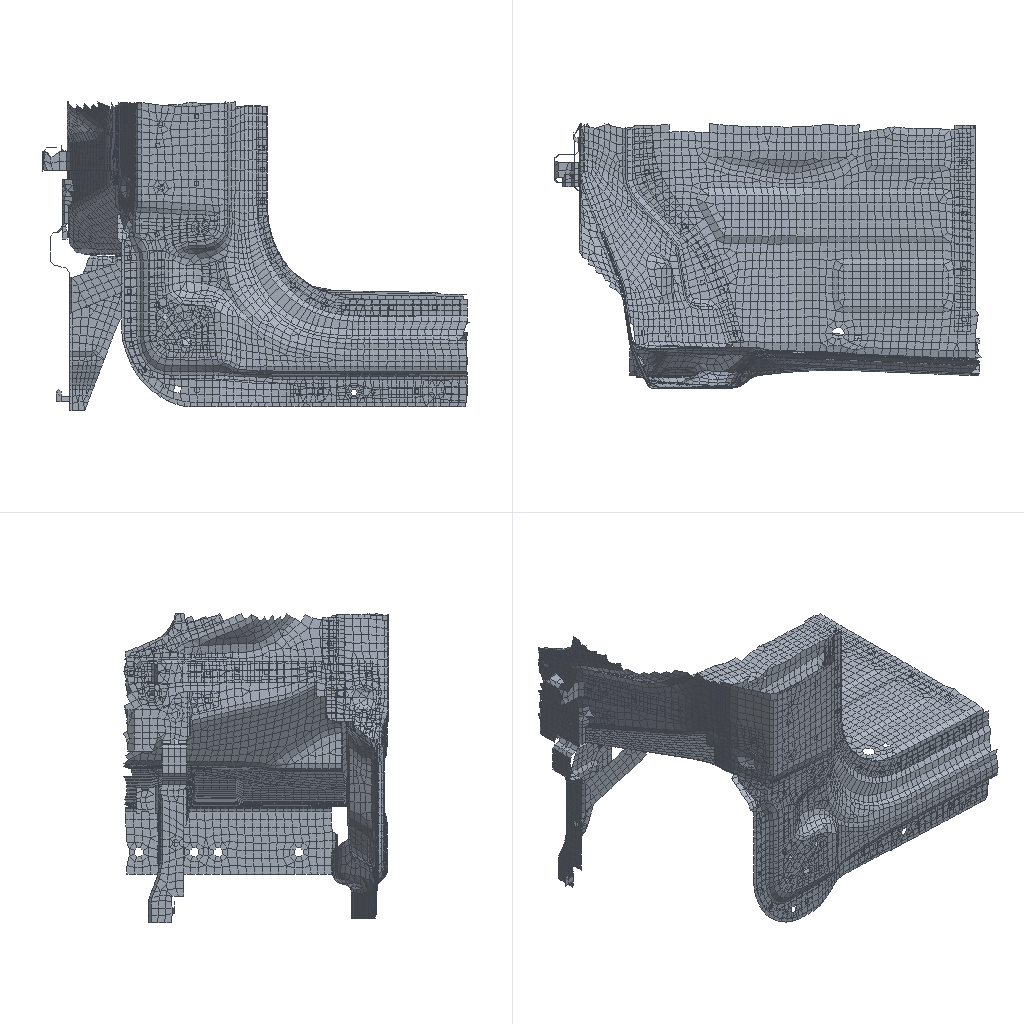Simulation study | nastran
Set-up summary:
category,name,step,type,value,unit,region
solver,nx_nastran
units,not stated in the deck,,not stated
analysis,deck,,static,static
analysis,solution,,SOL,101
load_step,SUBCASE 2,2,SUBCASE,SPC=2 LOAD=4
load_step,SUBCASE 3,3,SUBCASE,SPC=2 LOAD=3
load_step,requested,,,2
mesh,nodes,,,10089
mesh,elements,,,8887
element_type,CHEXA,,solid,95
element_type,CQUAD4,,shell,8185
element_type,CTRIA3,,shell,607
load,load commands in deck,,count,2
bc,support commands in deck,,count,747
check,setup vs results,,match,"every grid point's frame and coordinates and every element id; grid points of CHEXA, CQUAD4, CTRIA3 elements"
Nastran input file, long lists of numbers shortened:
$$------------------------------------------------------------------------------$
$$                                                                              $
$$ NASTRAN Input Deck Generated by HyperMesh Version  :10.0buil                 $
$$ Generated using HyperMesh-Nastran Template Version : 10.0build60
$$                                                                              $
$$   Template:  general                                                         $
$$                                                                              $
$$------------------------------------------------------------------------------$
$$------------------------------------------------------------------------------$
$$                      Executive Control Cards                                 $
$$------------------------------------------------------------------------------$
SOL 101
CEND
$$------------------------------------------------------------------------------$
$$                      Case Control Cards                                      $
$$------------------------------------------------------------------------------$
  DISPLACEMENT = ALL
  ESE = ALL
$
$HMNAME LOADSTEP               2"fy"
SUBCASE       2
  LABEL=   fy
  SPC =        2
  LOAD =        4
$
$HMNAME LOADSTEP               3"fx"
SUBCASE       3
  LABEL=   fx
  SPC =        2
  LOAD =        3
$$------------------------------------------------------------------------------$
$$                      Bulk Data Cards                                         $
$$------------------------------------------------------------------------------$
BEGIN BULK
PARAM,POST,-1
$$
$$  GRID Data
$$
GRID         650        -984.642-1013.18285.5856
GRID         651        -979.868-1013.43293.8012
$ (10087 more lines like these left out)
$$
$$  SPOINT Data
$$
$$
$$------------------------------------------------------------------------------$
$$             Group Definitions                                                $
$$------------------------------------------------------------------------------$
$$
$$ RBE2 Elements - Multiple dependent nodes
$$
RBE2     101835984101680  123456  616242  616243  616280  616281  616367+
+         616373  616374  616381  616382  616390  616391  616399  616401+
+         616409  616412  616421  616423  616431  616433  616440  616442+
+         616447  616495  616496  616522  616523  616550  616552  616857+
+         616923  616974  616976  616979  616981  617110  617387  617388+
+         618693  618714  618767  618768  618770  626113  626168  640699+
+         640712  642949  643271  646024  646046  646113  646130  646131+
+         646476  646477  646486  646488  646489  646490  646491  646517+
+         646521  646534  646535  646657  646658  646696  647133  647138+
+         647141  647143  647144  647147  648339  648382  648900  648931+
+         648933  648934 3749127 3749128 3749569 3749602 3749603 3749694+
+        3749714 3749733 3749734 3749740 3751159 3751160 3751162 3752617+
+        3752619 3752621 3752665 3752666 3752667 3752668 3752669 3752684+
+        3752690 3752691 3752694 3752695 3752698 3752699 3752701 3752702+
+        3752704 3754665 3754790 3754793 3754794 3754813 3754817 3754825+
+        3754835 3754844 3755010 3755011 3755012 3755013 3755038 3755048+
+        3755049 3755050 3755056 3755058 3755059 3755060 3755070 3755072+
+
$
$HMMOVE 84022697
$        1018359
$
$
$  RBE3 Elements
$
RBE3      326949         3756052  1234560.006546     123 37249890.005342+
+            123 37249920.444033     123 37249880.544079     123 3724985
RBE3      326950         3756053  1234561.94E-04     123 37249860.005865+
+            123 37249890.962111     123 37249850.03183      123 3724981
$ (1522 more lines like these left out)
$
$HMMOVE 57005012
$         326949THRU      326952  326954THRU      326961  326963THRU      326970
$         326972THRU      326979  326981THRU      326988  326990THRU      326997
$ (45 more lines like these left out)
CTRIA3    170731      13   87257   87311   87267
CTRIA3    170735      13   87254   87255   87266
$ (605 more lines like these left out)
$
$HMMOVE       18
$         170731  170735  170737THRU      170738  170742  170748  170751  170762
$         195368  195423  198996THRU      198997
$ (93 more lines like these left out)
CQUAD4    170729      13   87267   87311   87259   87260
CQUAD4    170730      13   87264   87267   87260   87261
$ (8183 more lines like these left out)
$
$HMMOVE       18
$         170729THRU      170730  170732THRU      170734  170736  170739THRU
$         170741  170743THRU      170747  170749THRU      170750  170752THRU
$ (264 more lines like these left out)
CHEXA     326953      10 3756052 3756055 3756054 3756053 3756056 3756059+
+        3756058 3756057
CHEXA     326962      10 3756061 3756064 3756063 3756062 3756065 3756068+
+        3756067 3756066
$ (186 more lines like these left out)
$
$HMMOVE 57005011
$         326953  326962  326971  326980  326989  326998  327007  327016  327691
$         327700  327925  327934  328141  328150  329689  329698  329707  329716
$ (89 more lines like these left out)
PSHELL         1       10.8            1               1
$
$HMNAME PROP                   2"120T" 4
$HWCOLOR PROP                  2       4
PSHELL         2       11.2            1               1
$
$HMNAME PROP                   3"100T" 4
$HWCOLOR PROP                  3       5
PSHELL         3       11.0            1               1
$
$HMNAME PROP                   4"150T" 4
$HWCOLOR PROP                  4       6
PSHELL         4       11.5            1               1
$
$HMNAME PROP                   8"200T" 4
$HWCOLOR PROP                  8      13
PSHELL         8       12.0            1               1
$
$HMNAME PROP                  10"180T" 4
$HWCOLOR PROP                 10      20
PSHELL        10       11.8            1               1
$
$
$
$HMNAME PROP                  11"80" 4
$HWCOLOR PROP                 11       3
PSHELL        11       20.8            2               2
$
$HMNAME PROP                  12"120" 4
$HWCOLOR PROP                 12       3
PSHELL        12       21.2            2               2
$
$HMNAME PROP                  13"180" 4
$HWCOLOR PROP                 13       3
PSHELL        13       21.8            2               2
$
$HMNAME PROP                  14"100" 4
$HWCOLOR PROP                 14       3
PSHELL        14       21.0            2               2
$
$HMNAME PROP                   5"150" 4
$HWCOLOR PROP                  5       3
PSHELL         5       21.5            2               2
$
$HMNAME PROP                   6"250" 4
$HWCOLOR PROP                  6       3
PSHELL         6       22.5            2               2
$
$HMNAME PROP                   7"200" 4
$HWCOLOR PROP                  7       3
PSHELL         7       22.0            2               2
$
$HMNAME PROP                  15"160" 4
$HWCOLOR PROP                 15       3
PSHELL        15       21.6            2               2
$$
$$  PSOLID Data
$
$HMNAME PROP                  15"spot" 5
$HWCOLOR PROP                 15      24
PSOLID        15       1
$
$HMNAME PROP                  10"spot.1" 5
$HWCOLOR PROP                 10       3
PSOLID        10       2
$$
$$------------------------------------------------------------------------------$
$$                      Material Definition Cards                               $
$$------------------------------------------------------------------------------$
$$--------------------------------------------------------------
$$ HYPERMESH TAGS
$$--------------------------------------------------------------
$$BEGIN TAGS
$$END TAGS
$$
$$  MAT1 Data
$
$HMNAME MAT                    1"steel" "MAT1"
$HWCOLOR MAT                   1       3
MAT1           1210000.0        0.3     7.90E-09
$
$HMNAME MAT                    2"steel.1" "MAT1"
$HWCOLOR MAT                   2       3
MAT1           2210000.0        0.3     7.80E-09
$$
$$
$$
$$------------------------------------------------------------------------------$
$ (39 more lines like these left out)
SPC            2 3638606  1234560.0
SPC            2 3638604  1234560.0
SPC            2 3638075  1234560.0
SPC            2 3638070  1234560.0
$ (743 more lines like these left out)
$$
$$  FORCE Data
$$
FORCE          384101680       01.0     500.0   0.0     0.0
FORCE          484101680       01.0     0.0     300.0   0.0
$HMASSEM       1       3 REAR_FLOOR
$HMASSEM_IDS    8402268984022694840226905100481151004311840226935100501051009711
$HMASSEM      28       4 5300010
$HMASSEM_IDS          18      20      21
$HMASSEM 5400100       7 sidebody_L
$HMASSEM_IDS    840226965400111054003010
$
ENDDATA
Results summary:
result,analysis,,,static
result,last_loadstep,,,2
result,primary field,,,displacements
result,max displacement,,,0.4904,model units